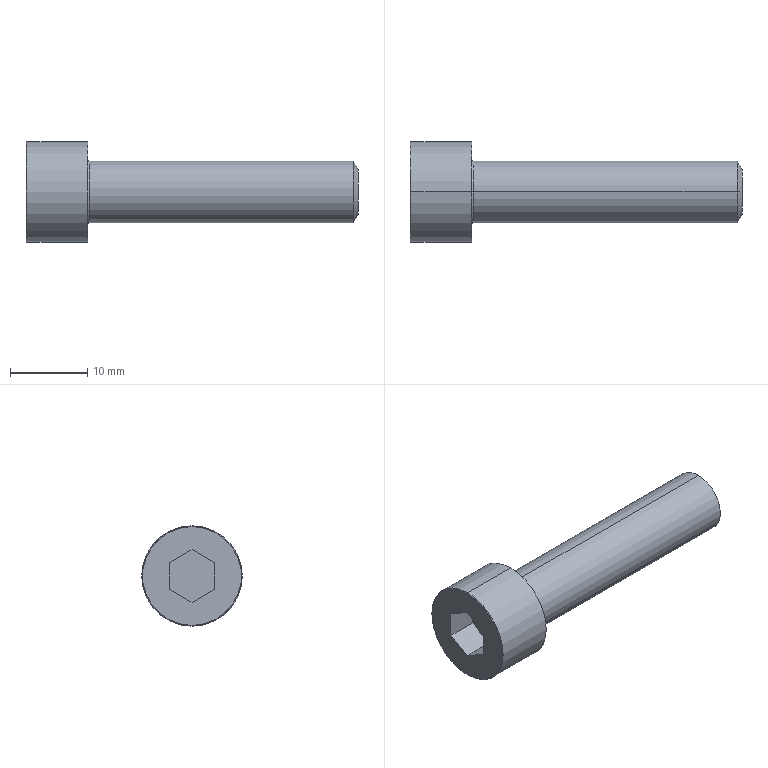Part | STEP file | 1 solid | 20 faces | box 43 x 13 x 13 mm | volume 2691 mm3 | plane 10 | torus 4 | cylinder 4 | cone 2 | commonest cylinder face diameters 8 x2 13 x2
STEP:
#1=CARTESIAN_POINT('',(0.,0.,6.4));
#2=VERTEX_POINT('',#1);
#3=CARTESIAN_POINT('',(0.,0.,-6.4));
#4=VERTEX_POINT('',#3);
#5=CARTESIAN_POINT('',(0.,0.,0.));
#6=DIRECTION('',(-1.,0.,0.));
#7=DIRECTION('',(0.,0.,-1.));
#8=AXIS2_PLACEMENT_3D('',#5,#6,#7);
#9=CIRCLE('',#8,6.4);
#10=EDGE_CURVE('',#2,#4,#9,.T.);
#11=ORIENTED_EDGE('',*,*,#10,.F.);
#12=CARTESIAN_POINT('',(0.1,0.,6.5));
#13=VERTEX_POINT('',#12);
#14=CARTESIAN_POINT('',(0.1,0.,6.4));
#15=DIRECTION('',(0.,1.,0.));
#16=DIRECTION('',(0.,0.,1.));
#17=AXIS2_PLACEMENT_3D('',#14,#15,#16);
#18=CIRCLE('',#17,0.1);
#19=EDGE_CURVE('',#2,#13,#18,.T.);
#20=ORIENTED_EDGE('',*,*,#19,.T.);
#21=CARTESIAN_POINT('',(0.1,0.,-6.5));
#22=VERTEX_POINT('',#21);
#23=CARTESIAN_POINT('',(0.1,0.,0.));
#24=DIRECTION('',(1.,0.,0.));
#25=DIRECTION('',(0.,0.,-1.));
#26=AXIS2_PLACEMENT_3D('',#23,#24,#25);
#27=CIRCLE('',#26,6.5);
#28=EDGE_CURVE('',#22,#13,#27,.T.);
#29=ORIENTED_EDGE('',*,*,#28,.F.);
#30=CARTESIAN_POINT('',(0.1,0.,-6.4));
#31=DIRECTION('',(0.,-1.,0.));
#32=DIRECTION('',(0.,0.,-1.));
#33=AXIS2_PLACEMENT_3D('',#30,#31,#32);
#34=CIRCLE('',#33,0.1);
#35=EDGE_CURVE('',#4,#22,#34,.T.);
#36=ORIENTED_EDGE('',*,*,#35,.F.);
#37=EDGE_LOOP('',(#11,#20,#29,#36));
#38=FACE_OUTER_BOUND('',#37,.T.);
#39=CARTESIAN_POINT('',(0.1,0.,0.));
#40=DIRECTION('',(1.,0.,0.));
#41=DIRECTION('',(0.,0.,-1.));
#42=AXIS2_PLACEMENT_3D('',#39,#40,#41);
#43=TOROIDAL_SURFACE('',#42,6.4,0.1);
#44=ADVANCED_FACE('',(#38),#43,.T.);
#45=CARTESIAN_POINT('',(43.,0.,2.917));
#46=VERTEX_POINT('',#45);
#47=CARTESIAN_POINT('',(43.,0.,-2.917));
#48=VERTEX_POINT('',#47);
#49=CARTESIAN_POINT('',(43.,0.,0.));
#50=DIRECTION('',(-1.,0.,0.));
#51=DIRECTION('',(0.,0.,1.));
#52=AXIS2_PLACEMENT_3D('',#49,#50,#51);
#53=CIRCLE('',#52,2.917);
#54=EDGE_CURVE('',#46,#48,#53,.T.);
#55=ORIENTED_EDGE('',*,*,#54,.T.);
#56=CARTESIAN_POINT('',(42.375,0.,-4.));
#57=VERTEX_POINT('',#56);
#58=CARTESIAN_POINT('',(42.375,0.,-4.));
#59=DIRECTION('',(-0.5,0.,-0.866));
#60=VECTOR('',#59,1000.);
#61=LINE('',#58,#60);
#62=EDGE_CURVE('',#48,#57,#61,.T.);
#63=ORIENTED_EDGE('',*,*,#62,.T.);
#64=CARTESIAN_POINT('',(42.375,0.,4.));
#65=VERTEX_POINT('',#64);
#66=CARTESIAN_POINT('',(42.375,0.,0.));
#67=DIRECTION('',(-1.,0.,0.));
#68=DIRECTION('',(0.,0.,1.));
#69=AXIS2_PLACEMENT_3D('',#66,#67,#68);
#70=CIRCLE('',#69,4.);
#71=EDGE_CURVE('',#65,#57,#70,.T.);
#72=ORIENTED_EDGE('',*,*,#71,.F.);
#73=CARTESIAN_POINT('',(42.375,0.,4.));
#74=DIRECTION('',(-0.5,0.,0.866));
#75=VECTOR('',#74,1000.);
#76=LINE('',#73,#75);
#77=EDGE_CURVE('',#46,#65,#76,.T.);
#78=ORIENTED_EDGE('',*,*,#77,.F.);
#79=EDGE_LOOP('',(#55,#63,#72,#78));
#80=FACE_OUTER_BOUND('',#79,.T.);
#81=CARTESIAN_POINT('',(42.375,0.,0.));
#82=DIRECTION('',(-1.,0.,0.));
#83=DIRECTION('',(0.,0.,1.));
#84=AXIS2_PLACEMENT_3D('',#81,#82,#83);
#85=CONICAL_SURFACE('',#84,4.,1.047);
#86=ADVANCED_FACE('',(#80),#85,.T.);
#87=CARTESIAN_POINT('',(8.,0.,-4.2));
#88=VERTEX_POINT('',#87);
#89=CARTESIAN_POINT('',(8.,0.,4.2));
#90=VERTEX_POINT('',#89);
#91=CARTESIAN_POINT('',(8.,0.,0.));
#92=DIRECTION('',(-1.,0.,0.));
#93=DIRECTION('',(0.,0.,1.));
#94=AXIS2_PLACEMENT_3D('',#91,#92,#93);
#95=CIRCLE('',#94,4.2);
#96=EDGE_CURVE('',#88,#90,#95,.T.);
#97=ORIENTED_EDGE('',*,*,#96,.F.);
#98=CARTESIAN_POINT('',(8.2,0.,-4.));
#99=VERTEX_POINT('',#98);
#100=CARTESIAN_POINT('',(8.2,0.,-4.2));
#101=DIRECTION('',(0.,1.,0.));
#102=DIRECTION('',(0.,0.,1.));
#103=AXIS2_PLACEMENT_3D('',#100,#101,#102);
#104=CIRCLE('',#103,0.2);
#105=EDGE_CURVE('',#88,#99,#104,.T.);
#106=ORIENTED_EDGE('',*,*,#105,.T.);
#107=CARTESIAN_POINT('',(8.2,0.,4.));
#108=VERTEX_POINT('',#107);
#109=CARTESIAN_POINT('',(8.2,0.,0.));
#110=DIRECTION('',(-1.,0.,0.));
#111=DIRECTION('',(0.,0.,1.));
#112=AXIS2_PLACEMENT_3D('',#109,#110,#111);
#113=CIRCLE('',#112,4.);
#114=EDGE_CURVE('',#99,#108,#113,.T.);
#115=ORIENTED_EDGE('',*,*,#114,.T.);
#116=CARTESIAN_POINT('',(8.2,0.,4.2));
#117=DIRECTION('',(0.,-1.,0.));
#118=DIRECTION('',(0.,0.,-1.));
#119=AXIS2_PLACEMENT_3D('',#116,#117,#118);
#120=CIRCLE('',#119,0.2);
#121=EDGE_CURVE('',#90,#108,#120,.T.);
#122=ORIENTED_EDGE('',*,*,#121,.F.);
#123=EDGE_LOOP('',(#97,#106,#115,#122));
#124=FACE_OUTER_BOUND('',#123,.T.);
#125=CARTESIAN_POINT('',(8.2,0.,0.));
#126=DIRECTION('',(-1.,0.,0.));
#127=DIRECTION('',(0.,0.,1.));
#128=AXIS2_PLACEMENT_3D('',#125,#126,#127);
#129=TOROIDAL_SURFACE('',#128,4.2,0.2);
#130=ADVANCED_FACE('',(#124),#129,.F.);
#131=CARTESIAN_POINT('',(8.,0.,6.5));
#132=VERTEX_POINT('',#131);
#133=CARTESIAN_POINT('',(8.,0.,-6.5));
#134=VERTEX_POINT('',#133);
#135=CARTESIAN_POINT('',(8.,0.,0.));
#136=DIRECTION('',(-1.,0.,0.));
#137=DIRECTION('',(0.,0.,1.));
#138=AXIS2_PLACEMENT_3D('',#135,#136,#137);
#139=CIRCLE('',#138,6.5);
#140=EDGE_CURVE('',#132,#134,#139,.T.);
#141=ORIENTED_EDGE('',*,*,#140,.T.);
#142=CARTESIAN_POINT('',(0.,0.,-6.5));
#143=DIRECTION('',(-1.,0.,0.));
#144=VECTOR('',#143,1000.);
#145=LINE('',#142,#144);
#146=EDGE_CURVE('',#134,#22,#145,.T.);
#147=ORIENTED_EDGE('',*,*,#146,.T.);
#148=ORIENTED_EDGE('',*,*,#28,.T.);
#149=CARTESIAN_POINT('',(0.,0.,6.5));
#150=DIRECTION('',(-1.,0.,0.));
#151=VECTOR('',#150,1000.);
#152=LINE('',#149,#151);
#153=EDGE_CURVE('',#132,#13,#152,.T.);
#154=ORIENTED_EDGE('',*,*,#153,.F.);
#155=EDGE_LOOP('',(#141,#147,#148,#154));
#156=FACE_OUTER_BOUND('',#155,.T.);
#157=CARTESIAN_POINT('',(0.,0.,0.));
#158=DIRECTION('',(-1.,0.,0.));
#159=DIRECTION('',(0.,0.,1.));
#160=AXIS2_PLACEMENT_3D('',#157,#158,#159);
#161=CYLINDRICAL_SURFACE('',#160,6.5);
#162=ADVANCED_FACE('',(#156),#161,.T.);
#163=ORIENTED_EDGE('',*,*,#71,.T.);
#164=CARTESIAN_POINT('',(0.,0.,-4.));
#165=DIRECTION('',(-1.,0.,0.));
#166=VECTOR('',#165,1000.);
#167=LINE('',#164,#166);
#168=EDGE_CURVE('',#57,#99,#167,.T.);
#169=ORIENTED_EDGE('',*,*,#168,.T.);
#170=CARTESIAN_POINT('',(8.2,0.,0.));
#171=DIRECTION('',(-1.,0.,0.));
#172=DIRECTION('',(0.,0.,1.));
#173=AXIS2_PLACEMENT_3D('',#170,#171,#172);
#174=CIRCLE('',#173,4.);
#175=EDGE_CURVE('',#108,#99,#174,.T.);
#176=ORIENTED_EDGE('',*,*,#175,.F.);
#177=CARTESIAN_POINT('',(0.,0.,4.));
#178=DIRECTION('',(-1.,0.,0.));
#179=VECTOR('',#178,1000.);
#180=LINE('',#177,#179);
#181=EDGE_CURVE('',#65,#108,#180,.T.);
#182=ORIENTED_EDGE('',*,*,#181,.F.);
#183=EDGE_LOOP('',(#163,#169,#176,#182));
#184=FACE_OUTER_BOUND('',#183,.T.);
#185=CARTESIAN_POINT('',(0.,0.,0.));
#186=DIRECTION('',(-1.,0.,0.));
#187=DIRECTION('',(0.,0.,1.));
#188=AXIS2_PLACEMENT_3D('',#185,#186,#187);
#189=CYLINDRICAL_SURFACE('',#188,4.);
#190=ADVANCED_FACE('',(#184),#189,.T.);
#191=ORIENTED_EDGE('',*,*,#168,.F.);
#192=CARTESIAN_POINT('',(42.375,0.,0.));
#193=DIRECTION('',(-1.,0.,0.));
#194=DIRECTION('',(0.,0.,1.));
#195=AXIS2_PLACEMENT_3D('',#192,#193,#194);
#196=CIRCLE('',#195,4.);
#197=EDGE_CURVE('',#57,#65,#196,.T.);
#198=ORIENTED_EDGE('',*,*,#197,.T.);
#199=ORIENTED_EDGE('',*,*,#181,.T.);
#200=ORIENTED_EDGE('',*,*,#114,.F.);
#201=EDGE_LOOP('',(#191,#198,#199,#200));
#202=FACE_OUTER_BOUND('',#201,.T.);
#203=CARTESIAN_POINT('',(0.,0.,0.));
#204=DIRECTION('',(-1.,0.,0.));
#205=DIRECTION('',(0.,0.,1.));
#206=AXIS2_PLACEMENT_3D('',#203,#204,#205);
#207=CYLINDRICAL_SURFACE('',#206,4.);
#208=ADVANCED_FACE('',(#202),#207,.T.);
#209=CARTESIAN_POINT('',(0.,0.,0.));
#210=DIRECTION('',(-1.,0.,0.));
#211=DIRECTION('',(0.,0.,-1.));
#212=AXIS2_PLACEMENT_3D('',#209,#210,#211);
#213=CIRCLE('',#212,6.4);
#214=EDGE_CURVE('',#4,#2,#213,.T.);
#215=ORIENTED_EDGE('',*,*,#214,.T.);
#216=ORIENTED_EDGE('',*,*,#10,.T.);
#217=EDGE_LOOP('',(#215,#216));
#218=FACE_OUTER_BOUND('',#217,.T.);
#219=CARTESIAN_POINT('',(0.,0.,3.43));
#220=VERTEX_POINT('',#219);
#221=CARTESIAN_POINT('',(0.,2.97,1.715));
#222=VERTEX_POINT('',#221);
#223=CARTESIAN_POINT('',(0.,0.,3.43));
#224=DIRECTION('',(0.,0.866,-0.5));
#225=VECTOR('',#224,1000.);
#226=LINE('',#223,#225);
#227=EDGE_CURVE('',#220,#222,#226,.T.);
#228=ORIENTED_EDGE('',*,*,#227,.F.);
#229=CARTESIAN_POINT('',(0.,-2.97,1.715));
#230=VERTEX_POINT('',#229);
#231=CARTESIAN_POINT('',(0.,-2.97,1.715));
#232=DIRECTION('',(0.,0.866,0.5));
#233=VECTOR('',#232,1000.);
#234=LINE('',#231,#233);
#235=EDGE_CURVE('',#230,#220,#234,.T.);
#236=ORIENTED_EDGE('',*,*,#235,.F.);
#237=CARTESIAN_POINT('',(0.,-2.97,-1.715));
#238=VERTEX_POINT('',#237);
#239=CARTESIAN_POINT('',(0.,-2.97,-1.715));
#240=DIRECTION('',(0.,0.,1.));
#241=VECTOR('',#240,1000.);
#242=LINE('',#239,#241);
#243=EDGE_CURVE('',#238,#230,#242,.T.);
#244=ORIENTED_EDGE('',*,*,#243,.F.);
#245=CARTESIAN_POINT('',(0.,0.,-3.43));
#246=VERTEX_POINT('',#245);
#247=CARTESIAN_POINT('',(0.,0.,-3.43));
#248=DIRECTION('',(0.,-0.866,0.5));
#249=VECTOR('',#248,1000.);
#250=LINE('',#247,#249);
#251=EDGE_CURVE('',#246,#238,#250,.T.);
#252=ORIENTED_EDGE('',*,*,#251,.F.);
#253=CARTESIAN_POINT('',(0.,2.97,-1.715));
#254=VERTEX_POINT('',#253);
#255=CARTESIAN_POINT('',(0.,2.97,-1.715));
#256=DIRECTION('',(0.,-0.866,-0.5));
#257=VECTOR('',#256,1000.);
#258=LINE('',#255,#257);
#259=EDGE_CURVE('',#254,#246,#258,.T.);
#260=ORIENTED_EDGE('',*,*,#259,.F.);
#261=CARTESIAN_POINT('',(0.,2.97,1.715));
#262=DIRECTION('',(0.,0.,-1.));
#263=VECTOR('',#262,1000.);
#264=LINE('',#261,#263);
#265=EDGE_CURVE('',#222,#254,#264,.T.);
#266=ORIENTED_EDGE('',*,*,#265,.F.);
#267=EDGE_LOOP('',(#228,#236,#244,#252,#260,#266));
#268=FACE_BOUND('',#267,.T.);
#269=CARTESIAN_POINT('',(0.,0.,0.));
#270=DIRECTION('',(1.,0.,0.));
#271=DIRECTION('',(0.,0.,-1.));
#272=AXIS2_PLACEMENT_3D('',#269,#270,#271);
#273=PLANE('',#272);
#274=ADVANCED_FACE('',(#218,#268),#273,.F.);
#275=ORIENTED_EDGE('',*,*,#146,.F.);
#276=CARTESIAN_POINT('',(8.,0.,0.));
#277=DIRECTION('',(-1.,0.,0.));
#278=DIRECTION('',(0.,0.,1.));
#279=AXIS2_PLACEMENT_3D('',#276,#277,#278);
#280=CIRCLE('',#279,6.5);
#281=EDGE_CURVE('',#134,#132,#280,.T.);
#282=ORIENTED_EDGE('',*,*,#281,.T.);
#283=ORIENTED_EDGE('',*,*,#153,.T.);
#284=CARTESIAN_POINT('',(0.1,0.,0.));
#285=DIRECTION('',(1.,0.,0.));
#286=DIRECTION('',(0.,0.,-1.));
#287=AXIS2_PLACEMENT_3D('',#284,#285,#286);
#288=CIRCLE('',#287,6.5);
#289=EDGE_CURVE('',#13,#22,#288,.T.);
#290=ORIENTED_EDGE('',*,*,#289,.T.);
#291=EDGE_LOOP('',(#275,#282,#283,#290));
#292=FACE_OUTER_BOUND('',#291,.T.);
#293=CARTESIAN_POINT('',(0.,0.,0.));
#294=DIRECTION('',(-1.,0.,0.));
#295=DIRECTION('',(0.,0.,1.));
#296=AXIS2_PLACEMENT_3D('',#293,#294,#295);
#297=CYLINDRICAL_SURFACE('',#296,6.5);
#298=ADVANCED_FACE('',(#292),#297,.T.);
#299=ORIENTED_EDGE('',*,*,#140,.F.);
#300=ORIENTED_EDGE('',*,*,#281,.F.);
#301=EDGE_LOOP('',(#299,#300));
#302=FACE_OUTER_BOUND('',#301,.T.);
#303=CARTESIAN_POINT('',(8.,0.,0.));
#304=DIRECTION('',(-1.,0.,0.));
#305=DIRECTION('',(0.,0.,1.));
#306=AXIS2_PLACEMENT_3D('',#303,#304,#305);
#307=CIRCLE('',#306,4.2);
#308=EDGE_CURVE('',#90,#88,#307,.T.);
#309=ORIENTED_EDGE('',*,*,#308,.T.);
#310=ORIENTED_EDGE('',*,*,#96,.T.);
#311=EDGE_LOOP('',(#309,#310));
#312=FACE_BOUND('',#311,.T.);
#313=CARTESIAN_POINT('',(8.,6.5,0.));
#314=DIRECTION('',(-1.,0.,0.));
#315=DIRECTION('',(0.,0.,1.));
#316=AXIS2_PLACEMENT_3D('',#313,#314,#315);
#317=PLANE('',#316);
#318=ADVANCED_FACE('',(#302,#312),#317,.F.);
#319=ORIENTED_EDGE('',*,*,#105,.F.);
#320=ORIENTED_EDGE('',*,*,#308,.F.);
#321=ORIENTED_EDGE('',*,*,#121,.T.);
#322=ORIENTED_EDGE('',*,*,#175,.T.);
#323=EDGE_LOOP('',(#319,#320,#321,#322));
#324=FACE_OUTER_BOUND('',#323,.T.);
#325=CARTESIAN_POINT('',(8.2,0.,0.));
#326=DIRECTION('',(-1.,0.,0.));
#327=DIRECTION('',(0.,0.,1.));
#328=AXIS2_PLACEMENT_3D('',#325,#326,#327);
#329=TOROIDAL_SURFACE('',#328,4.2,0.2);
#330=ADVANCED_FACE('',(#324),#329,.F.);
#331=ORIENTED_EDGE('',*,*,#235,.T.);
#332=CARTESIAN_POINT('',(4.,0.,3.43));
#333=VERTEX_POINT('',#332);
#334=CARTESIAN_POINT('',(4.,0.,3.43));
#335=DIRECTION('',(-1.,0.,0.));
#336=VECTOR('',#335,1000.);
#337=LINE('',#334,#336);
#338=EDGE_CURVE('',#333,#220,#337,.T.);
#339=ORIENTED_EDGE('',*,*,#338,.F.);
#340=CARTESIAN_POINT('',(4.,-2.97,1.715));
#341=VERTEX_POINT('',#340);
#342=CARTESIAN_POINT('',(4.,-2.97,1.715));
#343=DIRECTION('',(0.,0.866,0.5));
#344=VECTOR('',#343,1000.);
#345=LINE('',#342,#344);
#346=EDGE_CURVE('',#341,#333,#345,.T.);
#347=ORIENTED_EDGE('',*,*,#346,.F.);
#348=CARTESIAN_POINT('',(4.,-2.97,1.715));
#349=DIRECTION('',(-1.,0.,0.));
#350=VECTOR('',#349,1000.);
#351=LINE('',#348,#350);
#352=EDGE_CURVE('',#341,#230,#351,.T.);
#353=ORIENTED_EDGE('',*,*,#352,.T.);
#354=EDGE_LOOP('',(#331,#339,#347,#353));
#355=FACE_OUTER_BOUND('',#354,.T.);
#356=CARTESIAN_POINT('',(4.,-2.97,1.715));
#357=DIRECTION('',(0.,-0.5,0.866));
#358=DIRECTION('',(0.,-0.866,-0.5));
#359=AXIS2_PLACEMENT_3D('',#356,#357,#358);
#360=PLANE('',#359);
#361=ADVANCED_FACE('',(#355),#360,.F.);
#362=ORIENTED_EDGE('',*,*,#243,.T.);
#363=ORIENTED_EDGE('',*,*,#352,.F.);
#364=CARTESIAN_POINT('',(4.,-2.97,-1.715));
#365=VERTEX_POINT('',#364);
#366=CARTESIAN_POINT('',(4.,-2.97,-1.715));
#367=DIRECTION('',(0.,0.,1.));
#368=VECTOR('',#367,1000.);
#369=LINE('',#366,#368);
#370=EDGE_CURVE('',#365,#341,#369,.T.);
#371=ORIENTED_EDGE('',*,*,#370,.F.);
#372=CARTESIAN_POINT('',(4.,-2.97,-1.715));
#373=DIRECTION('',(-1.,0.,0.));
#374=VECTOR('',#373,1000.);
#375=LINE('',#372,#374);
#376=EDGE_CURVE('',#365,#238,#375,.T.);
#377=ORIENTED_EDGE('',*,*,#376,.T.);
#378=EDGE_LOOP('',(#362,#363,#371,#377));
#379=FACE_OUTER_BOUND('',#378,.T.);
#380=CARTESIAN_POINT('',(4.,-2.97,-1.715));
#381=DIRECTION('',(0.,-1.,0.));
#382=DIRECTION('',(0.,0.,-1.));
#383=AXIS2_PLACEMENT_3D('',#380,#381,#382);
#384=PLANE('',#383);
#385=ADVANCED_FACE('',(#379),#384,.F.);
#386=ORIENTED_EDGE('',*,*,#251,.T.);
#387=ORIENTED_EDGE('',*,*,#376,.F.);
#388=CARTESIAN_POINT('',(4.,0.,-3.43));
#389=VERTEX_POINT('',#388);
#390=CARTESIAN_POINT('',(4.,0.,-3.43));
#391=DIRECTION('',(0.,-0.866,0.5));
#392=VECTOR('',#391,1000.);
#393=LINE('',#390,#392);
#394=EDGE_CURVE('',#389,#365,#393,.T.);
#395=ORIENTED_EDGE('',*,*,#394,.F.);
#396=CARTESIAN_POINT('',(4.,0.,-3.43));
#397=DIRECTION('',(-1.,0.,0.));
#398=VECTOR('',#397,1000.);
#399=LINE('',#396,#398);
#400=EDGE_CURVE('',#389,#246,#399,.T.);
#401=ORIENTED_EDGE('',*,*,#400,.T.);
#402=EDGE_LOOP('',(#386,#387,#395,#401));
#403=FACE_OUTER_BOUND('',#402,.T.);
#404=CARTESIAN_POINT('',(4.,0.,-3.43));
#405=DIRECTION('',(0.,-0.5,-0.866));
#406=DIRECTION('',(0.,0.866,-0.5));
#407=AXIS2_PLACEMENT_3D('',#404,#405,#406);
#408=PLANE('',#407);
#409=ADVANCED_FACE('',(#403),#408,.F.);
#410=ORIENTED_EDGE('',*,*,#259,.T.);
#411=ORIENTED_EDGE('',*,*,#400,.F.);
#412=CARTESIAN_POINT('',(4.,2.97,-1.715));
#413=VERTEX_POINT('',#412);
#414=CARTESIAN_POINT('',(4.,2.97,-1.715));
#415=DIRECTION('',(0.,-0.866,-0.5));
#416=VECTOR('',#415,1000.);
#417=LINE('',#414,#416);
#418=EDGE_CURVE('',#413,#389,#417,.T.);
#419=ORIENTED_EDGE('',*,*,#418,.F.);
#420=CARTESIAN_POINT('',(4.,2.97,-1.715));
#421=DIRECTION('',(-1.,0.,0.));
#422=VECTOR('',#421,1000.);
#423=LINE('',#420,#422);
#424=EDGE_CURVE('',#413,#254,#423,.T.);
#425=ORIENTED_EDGE('',*,*,#424,.T.);
#426=EDGE_LOOP('',(#410,#411,#419,#425));
#427=FACE_OUTER_BOUND('',#426,.T.);
#428=CARTESIAN_POINT('',(4.,2.97,-1.715));
#429=DIRECTION('',(0.,0.5,-0.866));
#430=DIRECTION('',(0.,0.866,0.5));
#431=AXIS2_PLACEMENT_3D('',#428,#429,#430);
#432=PLANE('',#431);
#433=ADVANCED_FACE('',(#427),#432,.F.);
#434=ORIENTED_EDGE('',*,*,#265,.T.);
#435=ORIENTED_EDGE('',*,*,#424,.F.);
#436=CARTESIAN_POINT('',(4.,2.97,1.715));
#437=VERTEX_POINT('',#436);
#438=CARTESIAN_POINT('',(4.,2.97,1.715));
#439=DIRECTION('',(0.,0.,-1.));
#440=VECTOR('',#439,1000.);
#441=LINE('',#438,#440);
#442=EDGE_CURVE('',#437,#413,#441,.T.);
#443=ORIENTED_EDGE('',*,*,#442,.F.);
#444=CARTESIAN_POINT('',(4.,2.97,1.715));
#445=DIRECTION('',(-1.,0.,0.));
#446=VECTOR('',#445,1000.);
#447=LINE('',#444,#446);
#448=EDGE_CURVE('',#437,#222,#447,.T.);
#449=ORIENTED_EDGE('',*,*,#448,.T.);
#450=EDGE_LOOP('',(#434,#435,#443,#449));
#451=FACE_OUTER_BOUND('',#450,.T.);
#452=CARTESIAN_POINT('',(4.,2.97,1.715));
#453=DIRECTION('',(0.,1.,0.));
#454=DIRECTION('',(0.,0.,1.));
#455=AXIS2_PLACEMENT_3D('',#452,#453,#454);
#456=PLANE('',#455);
#457=ADVANCED_FACE('',(#451),#456,.F.);
#458=ORIENTED_EDGE('',*,*,#227,.T.);
#459=ORIENTED_EDGE('',*,*,#448,.F.);
#460=CARTESIAN_POINT('',(4.,0.,3.43));
#461=DIRECTION('',(0.,0.866,-0.5));
#462=VECTOR('',#461,1000.);
#463=LINE('',#460,#462);
#464=EDGE_CURVE('',#333,#437,#463,.T.);
#465=ORIENTED_EDGE('',*,*,#464,.F.);
#466=ORIENTED_EDGE('',*,*,#338,.T.);
#467=EDGE_LOOP('',(#458,#459,#465,#466));
#468=FACE_OUTER_BOUND('',#467,.T.);
#469=CARTESIAN_POINT('',(4.,0.,3.43));
#470=DIRECTION('',(0.,0.5,0.866));
#471=DIRECTION('',(0.,-0.866,0.5));
#472=AXIS2_PLACEMENT_3D('',#469,#470,#471);
#473=PLANE('',#472);
#474=ADVANCED_FACE('',(#468),#473,.F.);
#475=ORIENTED_EDGE('',*,*,#346,.T.);
#476=ORIENTED_EDGE('',*,*,#464,.T.);
#477=ORIENTED_EDGE('',*,*,#442,.T.);
#478=ORIENTED_EDGE('',*,*,#418,.T.);
#479=ORIENTED_EDGE('',*,*,#394,.T.);
#480=ORIENTED_EDGE('',*,*,#370,.T.);
#481=EDGE_LOOP('',(#475,#476,#477,#478,#479,#480));
#482=FACE_OUTER_BOUND('',#481,.T.);
#483=CARTESIAN_POINT('',(4.,-2.97,1.715));
#484=DIRECTION('',(1.,0.,0.));
#485=DIRECTION('',(0.,0.,-1.));
#486=AXIS2_PLACEMENT_3D('',#483,#484,#485);
#487=PLANE('',#486);
#488=ADVANCED_FACE('',(#482),#487,.F.);
#489=ORIENTED_EDGE('',*,*,#62,.F.);
#490=CARTESIAN_POINT('',(43.,0.,0.));
#491=DIRECTION('',(-1.,0.,0.));
#492=DIRECTION('',(0.,0.,1.));
#493=AXIS2_PLACEMENT_3D('',#490,#491,#492);
#494=CIRCLE('',#493,2.917);
#495=EDGE_CURVE('',#48,#46,#494,.T.);
#496=ORIENTED_EDGE('',*,*,#495,.T.);
#497=ORIENTED_EDGE('',*,*,#77,.T.);
#498=ORIENTED_EDGE('',*,*,#197,.F.);
#499=EDGE_LOOP('',(#489,#496,#497,#498));
#500=FACE_OUTER_BOUND('',#499,.T.);
#501=CARTESIAN_POINT('',(42.375,0.,0.));
#502=DIRECTION('',(-1.,0.,0.));
#503=DIRECTION('',(0.,0.,1.));
#504=AXIS2_PLACEMENT_3D('',#501,#502,#503);
#505=CONICAL_SURFACE('',#504,4.,1.047);
#506=ADVANCED_FACE('',(#500),#505,.T.);
#507=ORIENTED_EDGE('',*,*,#54,.F.);
#508=ORIENTED_EDGE('',*,*,#495,.F.);
#509=EDGE_LOOP('',(#507,#508));
#510=FACE_OUTER_BOUND('',#509,.T.);
#511=CARTESIAN_POINT('',(43.,4.,0.));
#512=DIRECTION('',(-1.,0.,0.));
#513=DIRECTION('',(0.,0.,1.));
#514=AXIS2_PLACEMENT_3D('',#511,#512,#513);
#515=PLANE('',#514);
#516=ADVANCED_FACE('',(#510),#515,.F.);
#517=ORIENTED_EDGE('',*,*,#19,.F.);
#518=ORIENTED_EDGE('',*,*,#214,.F.);
#519=ORIENTED_EDGE('',*,*,#35,.T.);
#520=ORIENTED_EDGE('',*,*,#289,.F.);
#521=EDGE_LOOP('',(#517,#518,#519,#520));
#522=FACE_OUTER_BOUND('',#521,.T.);
#523=CARTESIAN_POINT('',(0.1,0.,0.));
#524=DIRECTION('',(1.,0.,0.));
#525=DIRECTION('',(0.,0.,-1.));
#526=AXIS2_PLACEMENT_3D('',#523,#524,#525);
#527=TOROIDAL_SURFACE('',#526,6.4,0.1);
#528=ADVANCED_FACE('',(#522),#527,.T.);
#529=CLOSED_SHELL('',(#44,#86,#130,#162,#190,#208,#274,#298,#318,#330,#361,#385,#409,#433,#457,#474,#488,#506,#516,#528));
#530=MANIFOLD_SOLID_BREP('',#529);
#531=CARTESIAN_POINT('',(0.,0.,0.));
#532=DIRECTION('',(0.,0.,1.));
#533=DIRECTION('',(1.,0.,0.));
#534=AXIS2_PLACEMENT_3D('',#531,#532,#533);
#535=(LENGTH_UNIT()NAMED_UNIT(*)SI_UNIT(.MILLI.,.METRE.));
#536=UNCERTAINTY_MEASURE_WITH_UNIT(LENGTH_MEASURE(0.00001),#535,'','');
#537=(NAMED_UNIT(*)PLANE_ANGLE_UNIT()SI_UNIT($,.RADIAN.));
#538=(NAMED_UNIT(*)SI_UNIT($,.STERADIAN.)SOLID_ANGLE_UNIT());
#539=(GEOMETRIC_REPRESENTATION_CONTEXT(3)GLOBAL_UNCERTAINTY_ASSIGNED_CONTEXT((#536))GLOBAL_UNIT_ASSIGNED_CONTEXT((#535,#537,#538))REPRESENTATION_CONTEXT('',''));
#540=ADVANCED_BREP_SHAPE_REPRESENTATION('',(#530,#534),#539);